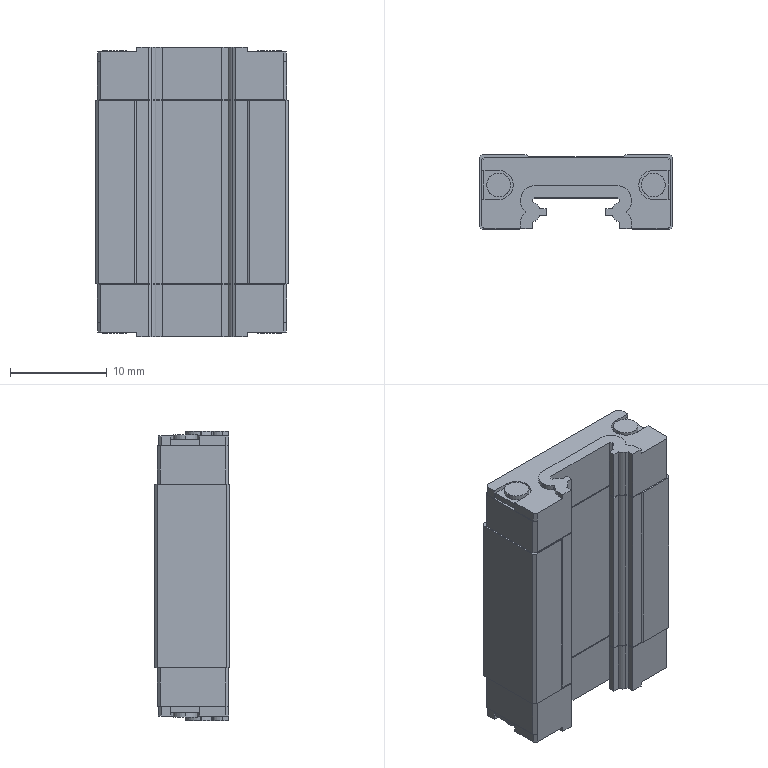Part | SolidWorks | features BaseBody 1 | 1 solid | 258 faces | box 20 x 7.8 x 30 mm | volume 3491 mm3 | plane 182 | cylinder 60 | cone 16 | commonest cylinder face diameters 2.2 x12 3 x10 2.1 x8 2.459 x8 2.5 x8 2.6 x8